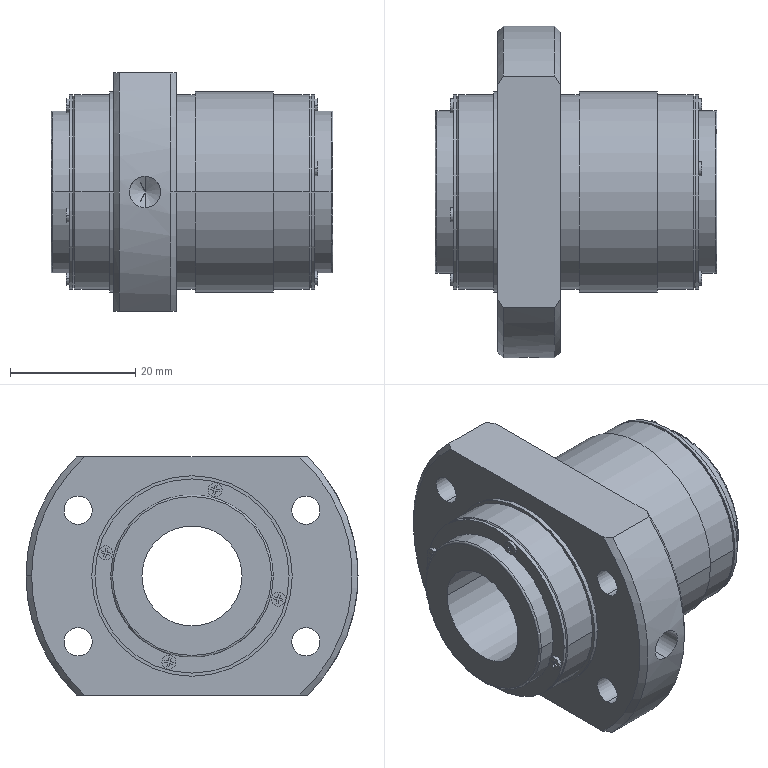Part | SolidWorks | features ICE 5, CirPattern 2, HoleWzd 2, Chamfer 1, Fillet 1, RevCut 1, Revolution 1 | 1 solid | 190 faces | box 45 x 53 x 38 mm | volume 34023 mm3 | plane 125 | cylinder 49 | cone 12 | torus 4 | commonest cylinder face diameters 2.24 x16 31 x10 4.5 x8 26 x4 32 x4 53 x3